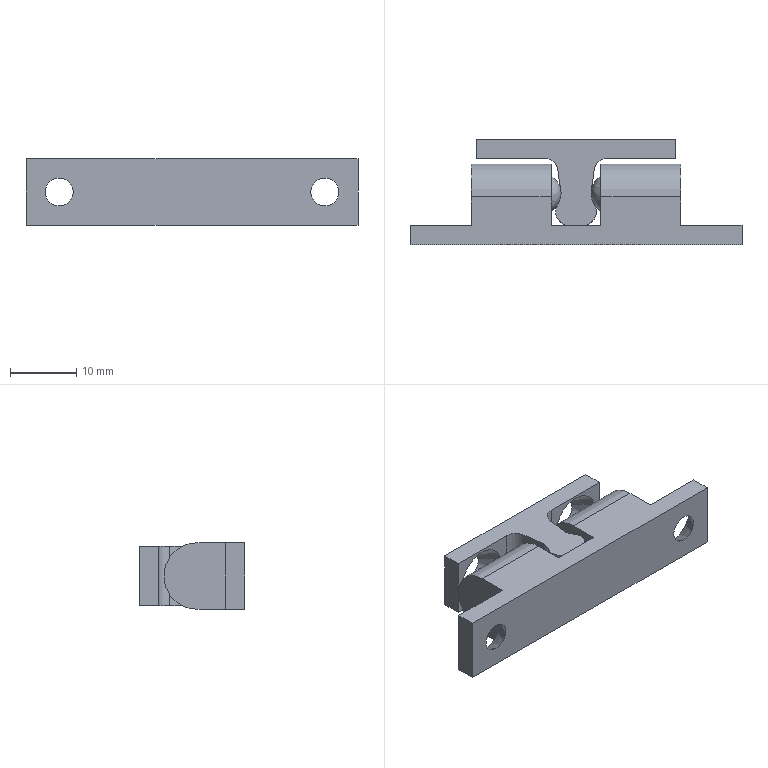Part | SolidWorks | features BaseBody 2 | 2 solids | 45 faces | box 50 x 15.9 x 10 mm | volume 4373 mm3 | plane 21 | cylinder 12 | cone 8 | spline 4 | commonest cylinder face diameters 6 x5 3.9 x3 4 x2 10 x2
STEP:
#1=CARTESIAN_POINT('',(-2.25,7.7,0.));
#2=VERTEX_POINT('',#1);
#3=CARTESIAN_POINT('',(-3.75,10.298,0.));
#4=VERTEX_POINT('',#3);
#5=CARTESIAN_POINT('',(-5.25,7.7,0.));
#6=DIRECTION('',(0.,0.,1.));
#7=DIRECTION('',(1.,0.,0.));
#8=AXIS2_PLACEMENT_3D('',#5,#6,#7);
#9=CIRCLE('',#8,3.);
#10=EDGE_CURVE('',#2,#4,#9,.T.);
#11=ORIENTED_EDGE('',*,*,#10,.F.);
#12=CARTESIAN_POINT('',(-3.75,5.102,0.));
#13=VERTEX_POINT('',#12);
#14=CARTESIAN_POINT('',(-5.25,7.7,0.));
#15=DIRECTION('',(0.,0.,-1.));
#16=DIRECTION('',(1.,0.,0.));
#17=AXIS2_PLACEMENT_3D('',#14,#15,#16);
#18=CIRCLE('',#17,3.);
#19=EDGE_CURVE('',#2,#13,#18,.T.);
#20=ORIENTED_EDGE('',*,*,#19,.T.);
#21=CARTESIAN_POINT('',(-3.75,7.7,0.));
#22=DIRECTION('',(-1.,0.,0.));
#23=DIRECTION('',(0.,0.,-1.));
#24=AXIS2_PLACEMENT_3D('',#21,#22,#23);
#25=CIRCLE('',#24,2.598);
#26=EDGE_CURVE('',#4,#13,#25,.T.);
#27=ORIENTED_EDGE('',*,*,#26,.F.);
#28=EDGE_LOOP('',(#11,#20,#27));
#29=FACE_OUTER_BOUND('',#28,.T.);
#30=CARTESIAN_POINT('',(-2.25,7.7,0.));
#31=CARTESIAN_POINT('',(-2.25,7.7,0.));
#32=CARTESIAN_POINT('',(-2.25,7.7,0.));
#33=CARTESIAN_POINT('',(-2.25,7.7,0.));
#34=CARTESIAN_POINT('',(-2.25,6.602,0.));
#35=CARTESIAN_POINT('',(-2.25,6.602,-2.196));
#36=CARTESIAN_POINT('',(-2.25,8.798,-2.196));
#37=CARTESIAN_POINT('',(-2.25,8.798,0.));
#38=CARTESIAN_POINT('',(-2.799,5.651,0.));
#39=CARTESIAN_POINT('',(-2.799,5.651,-4.098));
#40=CARTESIAN_POINT('',(-2.799,9.749,-4.098));
#41=CARTESIAN_POINT('',(-2.799,9.749,0.));
#42=CARTESIAN_POINT('',(-3.75,5.102,0.));
#43=CARTESIAN_POINT('',(-3.75,5.102,-5.196));
#44=CARTESIAN_POINT('',(-3.75,10.298,-5.196));
#45=CARTESIAN_POINT('',(-3.75,10.298,0.));
#46=(BOUNDED_SURFACE()B_SPLINE_SURFACE(3,3,((#30,#31,#32,#33),(#34,#35,#36,#37),(#38,#39,#40,#41),(#42,#43,#44,#45)),.UNSPECIFIED.,.F.,.F.,.F.)B_SPLINE_SURFACE_WITH_KNOTS((4,4),(4,4),(0.,1.),(0.,1.),.UNSPECIFIED.)GEOMETRIC_REPRESENTATION_ITEM()RATIONAL_B_SPLINE_SURFACE(((1.,0.3333,0.3333,1.),(0.9107,0.3036,0.3036,0.9107),(0.9107,0.3036,0.3036,0.9107),(1.,0.3333,0.3333,1.)))REPRESENTATION_ITEM('')SURFACE());
#47=ADVANCED_FACE('',(#29),#46,.T.);
#48=CARTESIAN_POINT('',(3.75,5.102,0.));
#49=VERTEX_POINT('',#48);
#50=CARTESIAN_POINT('',(3.75,10.298,0.));
#51=VERTEX_POINT('',#50);
#52=CARTESIAN_POINT('',(3.75,7.7,0.));
#53=DIRECTION('',(1.,0.,0.));
#54=DIRECTION('',(0.,0.,-1.));
#55=AXIS2_PLACEMENT_3D('',#52,#53,#54);
#56=CIRCLE('',#55,2.598);
#57=EDGE_CURVE('',#49,#51,#56,.T.);
#58=ORIENTED_EDGE('',*,*,#57,.F.);
#59=CARTESIAN_POINT('',(2.25,7.7,0.));
#60=VERTEX_POINT('',#59);
#61=CARTESIAN_POINT('',(5.25,7.7,0.));
#62=DIRECTION('',(0.,0.,-1.));
#63=DIRECTION('',(1.,0.,0.));
#64=AXIS2_PLACEMENT_3D('',#61,#62,#63);
#65=CIRCLE('',#64,3.);
#66=EDGE_CURVE('',#49,#60,#65,.T.);
#67=ORIENTED_EDGE('',*,*,#66,.T.);
#68=CARTESIAN_POINT('',(5.25,7.7,0.));
#69=DIRECTION('',(0.,0.,1.));
#70=DIRECTION('',(1.,0.,0.));
#71=AXIS2_PLACEMENT_3D('',#68,#69,#70);
#72=CIRCLE('',#71,3.);
#73=EDGE_CURVE('',#51,#60,#72,.T.);
#74=ORIENTED_EDGE('',*,*,#73,.F.);
#75=EDGE_LOOP('',(#58,#67,#74));
#76=FACE_OUTER_BOUND('',#75,.T.);
#77=CARTESIAN_POINT('',(3.75,5.102,0.));
#78=CARTESIAN_POINT('',(3.75,5.102,-5.196));
#79=CARTESIAN_POINT('',(3.75,10.298,-5.196));
#80=CARTESIAN_POINT('',(3.75,10.298,0.));
#81=CARTESIAN_POINT('',(2.799,5.651,0.));
#82=CARTESIAN_POINT('',(2.799,5.651,-4.098));
#83=CARTESIAN_POINT('',(2.799,9.749,-4.098));
#84=CARTESIAN_POINT('',(2.799,9.749,0.));
#85=CARTESIAN_POINT('',(2.25,6.602,0.));
#86=CARTESIAN_POINT('',(2.25,6.602,-2.196));
#87=CARTESIAN_POINT('',(2.25,8.798,-2.196));
#88=CARTESIAN_POINT('',(2.25,8.798,0.));
#89=CARTESIAN_POINT('',(2.25,7.7,0.));
#90=CARTESIAN_POINT('',(2.25,7.7,0.));
#91=CARTESIAN_POINT('',(2.25,7.7,0.));
#92=CARTESIAN_POINT('',(2.25,7.7,0.));
#93=(BOUNDED_SURFACE()B_SPLINE_SURFACE(3,3,((#77,#78,#79,#80),(#81,#82,#83,#84),(#85,#86,#87,#88),(#89,#90,#91,#92)),.UNSPECIFIED.,.F.,.F.,.T.)B_SPLINE_SURFACE_WITH_KNOTS((4,4),(4,4),(0.,1.),(0.,1.),.UNSPECIFIED.)GEOMETRIC_REPRESENTATION_ITEM()RATIONAL_B_SPLINE_SURFACE(((1.,0.3333,0.3333,1.),(0.9107,0.3036,0.3036,0.9107),(0.9107,0.3036,0.3036,0.9107),(1.,0.3333,0.3333,1.)))REPRESENTATION_ITEM('')SURFACE());
#94=ADVANCED_FACE('',(#76),#93,.T.);
#95=CARTESIAN_POINT('',(20.,0.,-2.1));
#96=VERTEX_POINT('',#95);
#97=CARTESIAN_POINT('',(20.,0.,2.1));
#98=VERTEX_POINT('',#97);
#99=CARTESIAN_POINT('',(20.,0.,0.));
#100=DIRECTION('',(0.,1.,0.));
#101=DIRECTION('',(0.,0.,1.));
#102=AXIS2_PLACEMENT_3D('',#99,#100,#101);
#103=CIRCLE('',#102,2.1);
#104=EDGE_CURVE('',#96,#98,#103,.T.);
#105=ORIENTED_EDGE('',*,*,#104,.F.);
#106=CARTESIAN_POINT('',(20.,2.9,-4.1));
#107=VERTEX_POINT('',#106);
#108=CARTESIAN_POINT('',(20.,2.9,-4.1));
#109=DIRECTION('',(0.,0.8232,-0.5677));
#110=VECTOR('',#109,1000.);
#111=LINE('',#108,#110);
#112=EDGE_CURVE('',#96,#107,#111,.T.);
#113=ORIENTED_EDGE('',*,*,#112,.T.);
#114=CARTESIAN_POINT('',(20.,2.9,4.1));
#115=VERTEX_POINT('',#114);
#116=CARTESIAN_POINT('',(20.,2.9,0.));
#117=DIRECTION('',(0.,-1.,0.));
#118=DIRECTION('',(0.,0.,1.));
#119=AXIS2_PLACEMENT_3D('',#116,#117,#118);
#120=CIRCLE('',#119,4.1);
#121=EDGE_CURVE('',#115,#107,#120,.T.);
#122=ORIENTED_EDGE('',*,*,#121,.F.);
#123=CARTESIAN_POINT('',(20.,2.9,4.1));
#124=DIRECTION('',(0.,0.8232,0.5677));
#125=VECTOR('',#124,1000.);
#126=LINE('',#123,#125);
#127=EDGE_CURVE('',#98,#115,#126,.T.);
#128=ORIENTED_EDGE('',*,*,#127,.F.);
#129=EDGE_LOOP('',(#105,#113,#122,#128));
#130=FACE_OUTER_BOUND('',#129,.T.);
#131=CARTESIAN_POINT('',(20.,2.9,0.));
#132=DIRECTION('',(0.,1.,0.));
#133=DIRECTION('',(0.,0.,1.));
#134=AXIS2_PLACEMENT_3D('',#131,#132,#133);
#135=CONICAL_SURFACE('',#134,4.1,0.6037);
#136=ADVANCED_FACE('',(#130),#135,.F.);
#137=CARTESIAN_POINT('',(-20.,0.,-2.1));
#138=VERTEX_POINT('',#137);
#139=CARTESIAN_POINT('',(-20.,0.,2.1));
#140=VERTEX_POINT('',#139);
#141=CARTESIAN_POINT('',(-20.,0.,0.));
#142=DIRECTION('',(0.,1.,0.));
#143=DIRECTION('',(0.,0.,1.));
#144=AXIS2_PLACEMENT_3D('',#141,#142,#143);
#145=CIRCLE('',#144,2.1);
#146=EDGE_CURVE('',#138,#140,#145,.T.);
#147=ORIENTED_EDGE('',*,*,#146,.F.);
#148=CARTESIAN_POINT('',(-20.,2.9,-4.1));
#149=VERTEX_POINT('',#148);
#150=CARTESIAN_POINT('',(-20.,2.9,-4.1));
#151=DIRECTION('',(0.,0.8232,-0.5677));
#152=VECTOR('',#151,1000.);
#153=LINE('',#150,#152);
#154=EDGE_CURVE('',#138,#149,#153,.T.);
#155=ORIENTED_EDGE('',*,*,#154,.T.);
#156=CARTESIAN_POINT('',(-20.,2.9,4.1));
#157=VERTEX_POINT('',#156);
#158=CARTESIAN_POINT('',(-20.,2.9,0.));
#159=DIRECTION('',(0.,-1.,0.));
#160=DIRECTION('',(0.,0.,1.));
#161=AXIS2_PLACEMENT_3D('',#158,#159,#160);
#162=CIRCLE('',#161,4.1);
#163=EDGE_CURVE('',#157,#149,#162,.T.);
#164=ORIENTED_EDGE('',*,*,#163,.F.);
#165=CARTESIAN_POINT('',(-20.,2.9,4.1));
#166=DIRECTION('',(0.,0.8232,0.5677));
#167=VECTOR('',#166,1000.);
#168=LINE('',#165,#167);
#169=EDGE_CURVE('',#140,#157,#168,.T.);
#170=ORIENTED_EDGE('',*,*,#169,.F.);
#171=EDGE_LOOP('',(#147,#155,#164,#170));
#172=FACE_OUTER_BOUND('',#171,.T.);
#173=CARTESIAN_POINT('',(-20.,2.9,0.));
#174=DIRECTION('',(0.,1.,0.));
#175=DIRECTION('',(0.,0.,1.));
#176=AXIS2_PLACEMENT_3D('',#173,#174,#175);
#177=CONICAL_SURFACE('',#176,4.1,0.6037);
#178=ADVANCED_FACE('',(#172),#177,.F.);
#179=CARTESIAN_POINT('',(25.,0.,5.));
#180=VERTEX_POINT('',#179);
#181=CARTESIAN_POINT('',(-25.,0.,5.));
#182=VERTEX_POINT('',#181);
#183=CARTESIAN_POINT('',(-25.,0.,5.));
#184=DIRECTION('',(-1.,0.,0.));
#185=VECTOR('',#184,1000.);
#186=LINE('',#183,#185);
#187=EDGE_CURVE('',#180,#182,#186,.T.);
#188=ORIENTED_EDGE('',*,*,#187,.T.);
#189=CARTESIAN_POINT('',(-25.,0.,-5.));
#190=VERTEX_POINT('',#189);
#191=CARTESIAN_POINT('',(-25.,0.,5.));
#192=DIRECTION('',(0.,0.,-1.));
#193=VECTOR('',#192,1000.);
#194=LINE('',#191,#193);
#195=EDGE_CURVE('',#182,#190,#194,.T.);
#196=ORIENTED_EDGE('',*,*,#195,.T.);
#197=CARTESIAN_POINT('',(25.,0.,-5.));
#198=VERTEX_POINT('',#197);
#199=CARTESIAN_POINT('',(-25.,0.,-5.));
#200=DIRECTION('',(1.,0.,0.));
#201=VECTOR('',#200,1000.);
#202=LINE('',#199,#201);
#203=EDGE_CURVE('',#190,#198,#202,.T.);
#204=ORIENTED_EDGE('',*,*,#203,.T.);
#205=CARTESIAN_POINT('',(25.,0.,5.));
#206=DIRECTION('',(0.,0.,1.));
#207=VECTOR('',#206,1000.);
#208=LINE('',#205,#207);
#209=EDGE_CURVE('',#198,#180,#208,.T.);
#210=ORIENTED_EDGE('',*,*,#209,.T.);
#211=EDGE_LOOP('',(#188,#196,#204,#210));
#212=FACE_OUTER_BOUND('',#211,.T.);
#213=CARTESIAN_POINT('',(20.,0.,0.));
#214=DIRECTION('',(0.,1.,0.));
#215=DIRECTION('',(0.,0.,1.));
#216=AXIS2_PLACEMENT_3D('',#213,#214,#215);
#217=CIRCLE('',#216,2.1);
#218=EDGE_CURVE('',#98,#96,#217,.T.);
#219=ORIENTED_EDGE('',*,*,#218,.T.);
#220=ORIENTED_EDGE('',*,*,#104,.T.);
#221=EDGE_LOOP('',(#219,#220));
#222=FACE_BOUND('',#221,.T.);
#223=CARTESIAN_POINT('',(-20.,0.,0.));
#224=DIRECTION('',(0.,1.,0.));
#225=DIRECTION('',(0.,0.,1.));
#226=AXIS2_PLACEMENT_3D('',#223,#224,#225);
#227=CIRCLE('',#226,2.1);
#228=EDGE_CURVE('',#140,#138,#227,.T.);
#229=ORIENTED_EDGE('',*,*,#228,.T.);
#230=ORIENTED_EDGE('',*,*,#146,.T.);
#231=EDGE_LOOP('',(#229,#230));
#232=FACE_BOUND('',#231,.T.);
#233=CARTESIAN_POINT('',(-25.,0.,5.));
#234=DIRECTION('',(0.,-1.,0.));
#235=DIRECTION('',(0.,0.,-1.));
#236=AXIS2_PLACEMENT_3D('',#233,#234,#235);
#237=PLANE('',#236);
#238=ADVANCED_FACE('',(#212,#222,#232),#237,.T.);
#239=CARTESIAN_POINT('',(-25.,2.9,5.));
#240=VERTEX_POINT('',#239);
#241=CARTESIAN_POINT('',(-25.,2.9,5.));
#242=DIRECTION('',(0.,1.,0.));
#243=VECTOR('',#242,1000.);
#244=LINE('',#241,#243);
#245=EDGE_CURVE('',#182,#240,#244,.T.);
#246=ORIENTED_EDGE('',*,*,#245,.T.);
#247=CARTESIAN_POINT('',(-25.,2.9,-5.));
#248=VERTEX_POINT('',#247);
#249=CARTESIAN_POINT('',(-25.,2.9,5.));
#250=DIRECTION('',(0.,0.,-1.));
#251=VECTOR('',#250,1000.);
#252=LINE('',#249,#251);
#253=EDGE_CURVE('',#240,#248,#252,.T.);
#254=ORIENTED_EDGE('',*,*,#253,.T.);
#255=CARTESIAN_POINT('',(-25.,2.9,-5.));
#256=DIRECTION('',(0.,-1.,0.));
#257=VECTOR('',#256,1000.);
#258=LINE('',#255,#257);
#259=EDGE_CURVE('',#248,#190,#258,.T.);
#260=ORIENTED_EDGE('',*,*,#259,.T.);
#261=ORIENTED_EDGE('',*,*,#195,.F.);
#262=EDGE_LOOP('',(#246,#254,#260,#261));
#263=FACE_OUTER_BOUND('',#262,.T.);
#264=CARTESIAN_POINT('',(-25.,2.9,5.));
#265=DIRECTION('',(-1.,0.,0.));
#266=DIRECTION('',(0.,0.,1.));
#267=AXIS2_PLACEMENT_3D('',#264,#265,#266);
#268=PLANE('',#267);
#269=ADVANCED_FACE('',(#263),#268,.T.);
#270=CARTESIAN_POINT('',(3.75,2.9,5.));
#271=VERTEX_POINT('',#270);
#272=CARTESIAN_POINT('',(-3.75,2.9,5.));
#273=VERTEX_POINT('',#272);
#274=CARTESIAN_POINT('',(0.,2.9,5.));
#275=DIRECTION('',(-1.,0.,0.));
#276=VECTOR('',#275,1000.);
#277=LINE('',#274,#276);
#278=EDGE_CURVE('',#271,#273,#277,.T.);
#279=ORIENTED_EDGE('',*,*,#278,.T.);
#280=CARTESIAN_POINT('',(-3.75,7.2,5.));
#281=VERTEX_POINT('',#280);
#282=CARTESIAN_POINT('',(-3.75,0.,5.));
#283=DIRECTION('',(0.,1.,0.));
#284=VECTOR('',#283,1000.);
#285=LINE('',#282,#284);
#286=EDGE_CURVE('',#273,#281,#285,.T.);
#287=ORIENTED_EDGE('',*,*,#286,.T.);
#288=CARTESIAN_POINT('',(-15.75,7.2,5.));
#289=VERTEX_POINT('',#288);
#290=CARTESIAN_POINT('',(0.,7.2,5.));
#291=DIRECTION('',(-1.,0.,0.));
#292=VECTOR('',#291,1000.);
#293=LINE('',#290,#292);
#294=EDGE_CURVE('',#281,#289,#293,.T.);
#295=ORIENTED_EDGE('',*,*,#294,.T.);
#296=CARTESIAN_POINT('',(-15.75,2.9,5.));
#297=VERTEX_POINT('',#296);
#298=CARTESIAN_POINT('',(-15.75,0.,5.));
#299=DIRECTION('',(0.,-1.,0.));
#300=VECTOR('',#299,1000.);
#301=LINE('',#298,#300);
#302=EDGE_CURVE('',#289,#297,#301,.T.);
#303=ORIENTED_EDGE('',*,*,#302,.T.);
#304=CARTESIAN_POINT('',(0.,2.9,5.));
#305=DIRECTION('',(-1.,0.,0.));
#306=VECTOR('',#305,1000.);
#307=LINE('',#304,#306);
#308=EDGE_CURVE('',#297,#240,#307,.T.);
#309=ORIENTED_EDGE('',*,*,#308,.T.);
#310=ORIENTED_EDGE('',*,*,#245,.F.);
#311=ORIENTED_EDGE('',*,*,#187,.F.);
#312=CARTESIAN_POINT('',(25.,2.9,5.));
#313=VERTEX_POINT('',#312);
#314=CARTESIAN_POINT('',(25.,0.,5.));
#315=DIRECTION('',(0.,1.,0.));
#316=VECTOR('',#315,1000.);
#317=LINE('',#314,#316);
#318=EDGE_CURVE('',#180,#313,#317,.T.);
#319=ORIENTED_EDGE('',*,*,#318,.T.);
#320=CARTESIAN_POINT('',(15.75,2.9,5.));
#321=VERTEX_POINT('',#320);
#322=CARTESIAN_POINT('',(0.,2.9,5.));
#323=DIRECTION('',(-1.,0.,0.));
#324=VECTOR('',#323,1000.);
#325=LINE('',#322,#324);
#326=EDGE_CURVE('',#313,#321,#325,.T.);
#327=ORIENTED_EDGE('',*,*,#326,.T.);
#328=CARTESIAN_POINT('',(15.75,7.2,5.));
#329=VERTEX_POINT('',#328);
#330=CARTESIAN_POINT('',(15.75,0.,5.));
#331=DIRECTION('',(0.,1.,0.));
#332=VECTOR('',#331,1000.);
#333=LINE('',#330,#332);
#334=EDGE_CURVE('',#321,#329,#333,.T.);
#335=ORIENTED_EDGE('',*,*,#334,.T.);
#336=CARTESIAN_POINT('',(3.75,7.2,5.));
#337=VERTEX_POINT('',#336);
#338=CARTESIAN_POINT('',(0.,7.2,5.));
#339=DIRECTION('',(-1.,0.,0.));
#340=VECTOR('',#339,1000.);
#341=LINE('',#338,#340);
#342=EDGE_CURVE('',#329,#337,#341,.T.);
#343=ORIENTED_EDGE('',*,*,#342,.T.);
#344=CARTESIAN_POINT('',(3.75,0.,5.));
#345=DIRECTION('',(0.,-1.,0.));
#346=VECTOR('',#345,1000.);
#347=LINE('',#344,#346);
#348=EDGE_CURVE('',#337,#271,#347,.T.);
#349=ORIENTED_EDGE('',*,*,#348,.T.);
#350=EDGE_LOOP('',(#279,#287,#295,#303,#309,#310,#311,#319,#327,#335,#343,#349));
#351=FACE_OUTER_BOUND('',#350,.T.);
#352=CARTESIAN_POINT('',(0.,0.,5.));
#353=DIRECTION('',(0.,0.,1.));
#354=DIRECTION('',(1.,0.,0.));
#355=AXIS2_PLACEMENT_3D('',#352,#353,#354);
#356=PLANE('',#355);
#357=ADVANCED_FACE('',(#351),#356,.T.);
#358=ORIENTED_EDGE('',*,*,#318,.F.);
#359=ORIENTED_EDGE('',*,*,#209,.F.);
#360=CARTESIAN_POINT('',(25.,2.9,-5.));
#361=VERTEX_POINT('',#360);
#362=CARTESIAN_POINT('',(25.,0.,-5.));
#363=DIRECTION('',(0.,1.,0.));
#364=VECTOR('',#363,1000.);
#365=LINE('',#362,#364);
#366=EDGE_CURVE('',#198,#361,#365,.T.);
#367=ORIENTED_EDGE('',*,*,#366,.T.);
#368=CARTESIAN_POINT('',(25.,2.9,5.));
#369=DIRECTION('',(0.,0.,1.));
#370=VECTOR('',#369,1000.);
#371=LINE('',#368,#370);
#372=EDGE_CURVE('',#361,#313,#371,.T.);
#373=ORIENTED_EDGE('',*,*,#372,.T.);
#374=EDGE_LOOP('',(#358,#359,#367,#373));
#375=FACE_OUTER_BOUND('',#374,.T.);
#376=CARTESIAN_POINT('',(25.,0.,5.));
#377=DIRECTION('',(1.,0.,0.));
#378=DIRECTION('',(0.,0.,-1.));
#379=AXIS2_PLACEMENT_3D('',#376,#377,#378);
#380=PLANE('',#379);
#381=ADVANCED_FACE('',(#375),#380,.T.);
#382=CARTESIAN_POINT('',(-3.75,2.9,-5.));
#383=VERTEX_POINT('',#382);
#384=CARTESIAN_POINT('',(-3.75,7.2,-5.));
#385=VERTEX_POINT('',#384);
#386=CARTESIAN_POINT('',(-3.75,0.,-5.));
#387=DIRECTION('',(0.,1.,0.));
#388=VECTOR('',#387,1000.);
#389=LINE('',#386,#388);
#390=EDGE_CURVE('',#383,#385,#389,.T.);
#391=ORIENTED_EDGE('',*,*,#390,.F.);
#392=CARTESIAN_POINT('',(3.75,2.9,-5.));
#393=VERTEX_POINT('',#392);
#394=CARTESIAN_POINT('',(0.,2.9,-5.));
#395=DIRECTION('',(-1.,0.,0.));
#396=VECTOR('',#395,1000.);
#397=LINE('',#394,#396);
#398=EDGE_CURVE('',#393,#383,#397,.T.);
#399=ORIENTED_EDGE('',*,*,#398,.F.);
#400=CARTESIAN_POINT('',(3.75,7.2,-5.));
#401=VERTEX_POINT('',#400);
#402=CARTESIAN_POINT('',(3.75,0.,-5.));
#403=DIRECTION('',(0.,-1.,0.));
#404=VECTOR('',#403,1000.);
#405=LINE('',#402,#404);
#406=EDGE_CURVE('',#401,#393,#405,.T.);
#407=ORIENTED_EDGE('',*,*,#406,.F.);
#408=CARTESIAN_POINT('',(15.75,7.2,-5.));
#409=VERTEX_POINT('',#408);
#410=CARTESIAN_POINT('',(0.,7.2,-5.));
#411=DIRECTION('',(-1.,0.,0.));
#412=VECTOR('',#411,1000.);
#413=LINE('',#410,#412);
#414=EDGE_CURVE('',#409,#401,#413,.T.);
#415=ORIENTED_EDGE('',*,*,#414,.F.);
#416=CARTESIAN_POINT('',(15.75,2.9,-5.));
#417=VERTEX_POINT('',#416);
#418=CARTESIAN_POINT('',(15.75,0.,-5.));
#419=DIRECTION('',(0.,1.,0.));
#420=VECTOR('',#419,1000.);
#421=LINE('',#418,#420);
#422=EDGE_CURVE('',#417,#409,#421,.T.);
#423=ORIENTED_EDGE('',*,*,#422,.F.);
#424=CARTESIAN_POINT('',(0.,2.9,-5.));
#425=DIRECTION('',(-1.,0.,0.));
#426=VECTOR('',#425,1000.);
#427=LINE('',#424,#426);
#428=EDGE_CURVE('',#361,#417,#427,.T.);
#429=ORIENTED_EDGE('',*,*,#428,.F.);
#430=ORIENTED_EDGE('',*,*,#366,.F.);
#431=ORIENTED_EDGE('',*,*,#203,.F.);
#432=ORIENTED_EDGE('',*,*,#259,.F.);
#433=CARTESIAN_POINT('',(-15.75,2.9,-5.));
#434=VERTEX_POINT('',#433);
#435=CARTESIAN_POINT('',(0.,2.9,-5.));
#436=DIRECTION('',(-1.,0.,0.));
#437=VECTOR('',#436,1000.);
#438=LINE('',#435,#437);
#439=EDGE_CURVE('',#434,#248,#438,.T.);
#440=ORIENTED_EDGE('',*,*,#439,.F.);
#441=CARTESIAN_POINT('',(-15.75,7.2,-5.));
#442=VERTEX_POINT('',#441);
#443=CARTESIAN_POINT('',(-15.75,0.,-5.));
#444=DIRECTION('',(0.,-1.,0.));
#445=VECTOR('',#444,1000.);
#446=LINE('',#443,#445);
#447=EDGE_CURVE('',#442,#434,#446,.T.);
#448=ORIENTED_EDGE('',*,*,#447,.F.);
#449=CARTESIAN_POINT('',(0.,7.2,-5.));
#450=DIRECTION('',(-1.,0.,0.));
#451=VECTOR('',#450,1000.);
#452=LINE('',#449,#451);
#453=EDGE_CURVE('',#385,#442,#452,.T.);
#454=ORIENTED_EDGE('',*,*,#453,.F.);
#455=EDGE_LOOP('',(#391,#399,#407,#415,#423,#429,#430,#431,#432,#440,#448,#454));
#456=FACE_OUTER_BOUND('',#455,.T.);
#457=CARTESIAN_POINT('',(0.,0.,-5.));
#458=DIRECTION('',(0.,0.,1.));
#459=DIRECTION('',(1.,0.,0.));
#460=AXIS2_PLACEMENT_3D('',#457,#458,#459);
#461=PLANE('',#460);
#462=ADVANCED_FACE('',(#456),#461,.F.);
#463=ORIENTED_EDGE('',*,*,#112,.F.);
#464=ORIENTED_EDGE('',*,*,#218,.F.);
#465=ORIENTED_EDGE('',*,*,#127,.T.);
#466=CARTESIAN_POINT('',(20.,2.9,0.));
#467=DIRECTION('',(0.,-1.,0.));
#468=DIRECTION('',(0.,0.,1.));
#469=AXIS2_PLACEMENT_3D('',#466,#467,#468);
#470=CIRCLE('',#469,4.1);
#471=EDGE_CURVE('',#107,#115,#470,.T.);
#472=ORIENTED_EDGE('',*,*,#471,.F.);
#473=EDGE_LOOP('',(#463,#464,#465,#472));
#474=FACE_OUTER_BOUND('',#473,.T.);
#475=CARTESIAN_POINT('',(20.,2.9,0.));
#476=DIRECTION('',(0.,1.,0.));
#477=DIRECTION('',(0.,0.,1.));
#478=AXIS2_PLACEMENT_3D('',#475,#476,#477);
#479=CONICAL_SURFACE('',#478,4.1,0.6037);
#480=ADVANCED_FACE('',(#474),#479,.F.);
#481=ORIENTED_EDGE('',*,*,#154,.F.);
#482=ORIENTED_EDGE('',*,*,#228,.F.);
#483=ORIENTED_EDGE('',*,*,#169,.T.);
#484=CARTESIAN_POINT('',(-20.,2.9,0.));
#485=DIRECTION('',(0.,-1.,0.));
#486=DIRECTION('',(0.,0.,1.));
#487=AXIS2_PLACEMENT_3D('',#484,#485,#486);
#488=CIRCLE('',#487,4.1);
#489=EDGE_CURVE('',#149,#157,#488,.T.);
#490=ORIENTED_EDGE('',*,*,#489,.F.);
#491=EDGE_LOOP('',(#481,#482,#483,#490));
#492=FACE_OUTER_BOUND('',#491,.T.);
#493=CARTESIAN_POINT('',(-20.,2.9,0.));
#494=DIRECTION('',(0.,1.,0.));
#495=DIRECTION('',(0.,0.,1.));
#496=AXIS2_PLACEMENT_3D('',#493,#494,#495);
#497=CONICAL_SURFACE('',#496,4.1,0.6037);
#498=ADVANCED_FACE('',(#492),#497,.F.);
#499=ORIENTED_EDGE('',*,*,#308,.F.);
#500=CARTESIAN_POINT('',(-15.75,2.9,5.));
#501=DIRECTION('',(0.,0.,-1.));
#502=VECTOR('',#501,1000.);
#503=LINE('',#500,#502);
#504=EDGE_CURVE('',#297,#434,#503,.T.);
#505=ORIENTED_EDGE('',*,*,#504,.T.);
#506=ORIENTED_EDGE('',*,*,#439,.T.);
#507=ORIENTED_EDGE('',*,*,#253,.F.);
#508=EDGE_LOOP('',(#499,#505,#506,#507));
#509=FACE_OUTER_BOUND('',#508,.T.);
#510=ORIENTED_EDGE('',*,*,#163,.T.);
#511=ORIENTED_EDGE('',*,*,#489,.T.);
#512=EDGE_LOOP('',(#510,#511));
#513=FACE_BOUND('',#512,.T.);
#514=CARTESIAN_POINT('',(-15.75,2.9,5.));
#515=DIRECTION('',(0.,1.,0.));
#516=DIRECTION('',(0.,0.,1.));
#517=AXIS2_PLACEMENT_3D('',#514,#515,#516);
#518=PLANE('',#517);
#519=ADVANCED_FACE('',(#509,#513),#518,.T.);
#520=CARTESIAN_POINT('',(-3.75,2.9,5.));
#521=DIRECTION('',(0.,0.,-1.));
#522=VECTOR('',#521,1000.);
#523=LINE('',#520,#522);
#524=EDGE_CURVE('',#273,#383,#523,.T.);
#525=ORIENTED_EDGE('',*,*,#524,.T.);
#526=ORIENTED_EDGE('',*,*,#390,.T.);
#527=CARTESIAN_POINT('',(-3.75,7.2,0.));
#528=DIRECTION('',(1.,0.,0.));
#529=DIRECTION('',(0.,0.,-1.));
#530=AXIS2_PLACEMENT_3D('',#527,#528,#529);
#531=CIRCLE('',#530,5.);
#532=EDGE_CURVE('',#385,#281,#531,.T.);
#533=ORIENTED_EDGE('',*,*,#532,.T.);
#534=ORIENTED_EDGE('',*,*,#286,.F.);
#535=EDGE_LOOP('',(#525,#526,#533,#534));
#536=FACE_OUTER_BOUND('',#535,.T.);
#537=ORIENTED_EDGE('',*,*,#26,.T.);
#538=CARTESIAN_POINT('',(-3.75,7.7,0.));
#539=DIRECTION('',(-1.,0.,0.));
#540=DIRECTION('',(0.,0.,-1.));
#541=AXIS2_PLACEMENT_3D('',#538,#539,#540);
#542=CIRCLE('',#541,2.598);
#543=EDGE_CURVE('',#13,#4,#542,.T.);
#544=ORIENTED_EDGE('',*,*,#543,.T.);
#545=EDGE_LOOP('',(#537,#544));
#546=FACE_BOUND('',#545,.T.);
#547=CARTESIAN_POINT('',(-3.75,2.9,5.));
#548=DIRECTION('',(1.,0.,0.));
#549=DIRECTION('',(0.,0.,-1.));
#550=AXIS2_PLACEMENT_3D('',#547,#548,#549);
#551=PLANE('',#550);
#552=ADVANCED_FACE('',(#536,#546),#551,.T.);
#553=ORIENTED_EDGE('',*,*,#278,.F.);
#554=CARTESIAN_POINT('',(3.75,2.9,5.));
#555=DIRECTION('',(0.,0.,-1.));
#556=VECTOR('',#555,1000.);
#557=LINE('',#554,#556);
#558=EDGE_CURVE('',#271,#393,#557,.T.);
#559=ORIENTED_EDGE('',*,*,#558,.T.);
#560=ORIENTED_EDGE('',*,*,#398,.T.);
#561=ORIENTED_EDGE('',*,*,#524,.F.);
#562=EDGE_LOOP('',(#553,#559,#560,#561));
#563=FACE_OUTER_BOUND('',#562,.T.);
#564=CARTESIAN_POINT('',(3.75,2.9,5.));
#565=DIRECTION('',(0.,1.,0.));
#566=DIRECTION('',(0.,0.,1.));
#567=AXIS2_PLACEMENT_3D('',#564,#565,#566);
#568=PLANE('',#567);
#569=ADVANCED_FACE('',(#563),#568,.T.);
#570=ORIENTED_EDGE('',*,*,#558,.F.);
#571=ORIENTED_EDGE('',*,*,#348,.F.);
#572=CARTESIAN_POINT('',(3.75,7.2,0.));
#573=DIRECTION('',(-1.,0.,0.));
#574=DIRECTION('',(0.,0.,-1.));
#575=AXIS2_PLACEMENT_3D('',#572,#573,#574);
#576=CIRCLE('',#575,5.);
#577=EDGE_CURVE('',#337,#401,#576,.T.);
#578=ORIENTED_EDGE('',*,*,#577,.T.);
#579=ORIENTED_EDGE('',*,*,#406,.T.);
#580=EDGE_LOOP('',(#570,#571,#578,#579));
#581=FACE_OUTER_BOUND('',#580,.T.);
#582=CARTESIAN_POINT('',(3.75,7.7,0.));
#583=DIRECTION('',(1.,0.,0.));
#584=DIRECTION('',(0.,0.,-1.));
#585=AXIS2_PLACEMENT_3D('',#582,#583,#584);
#586=CIRCLE('',#585,2.598);
#587=EDGE_CURVE('',#51,#49,#586,.T.);
#588=ORIENTED_EDGE('',*,*,#587,.T.);
#589=ORIENTED_EDGE('',*,*,#57,.T.);
#590=EDGE_LOOP('',(#588,#589));
#591=FACE_BOUND('',#590,.T.);
#592=CARTESIAN_POINT('',(3.75,12.2,5.));
#593=DIRECTION('',(-1.,0.,0.));
#594=DIRECTION('',(0.,-1.,0.));
#595=AXIS2_PLACEMENT_3D('',#592,#593,#594);
#596=PLANE('',#595);
#597=ADVANCED_FACE('',(#581,#591),#596,.T.);
#598=CARTESIAN_POINT('',(15.75,7.2,0.));
#599=DIRECTION('',(-1.,0.,0.));
#600=DIRECTION('',(0.,0.,-1.));
#601=AXIS2_PLACEMENT_3D('',#598,#599,#600);
#602=CIRCLE('',#601,5.);
#603=EDGE_CURVE('',#329,#409,#602,.T.);
#604=ORIENTED_EDGE('',*,*,#603,.T.);
#605=ORIENTED_EDGE('',*,*,#414,.T.);
#606=ORIENTED_EDGE('',*,*,#577,.F.);
#607=ORIENTED_EDGE('',*,*,#342,.F.);
#608=EDGE_LOOP('',(#604,#605,#606,#607));
#609=FACE_OUTER_BOUND('',#608,.T.);
#610=CARTESIAN_POINT('',(50.,7.2,0.));
#611=DIRECTION('',(1.,0.,0.));
#612=DIRECTION('',(0.,0.,-1.));
#613=AXIS2_PLACEMENT_3D('',#610,#611,#612);
#614=CYLINDRICAL_SURFACE('',#613,5.);
#615=ADVANCED_FACE('',(#609),#614,.T.);
#616=CARTESIAN_POINT('',(15.75,2.9,5.));
#617=DIRECTION('',(0.,0.,-1.));
#618=VECTOR('',#617,1000.);
#619=LINE('',#616,#618);
#620=EDGE_CURVE('',#321,#417,#619,.T.);
#621=ORIENTED_EDGE('',*,*,#620,.T.);
#622=ORIENTED_EDGE('',*,*,#422,.T.);
#623=ORIENTED_EDGE('',*,*,#603,.F.);
#624=ORIENTED_EDGE('',*,*,#334,.F.);
#625=EDGE_LOOP('',(#621,#622,#623,#624));
#626=FACE_OUTER_BOUND('',#625,.T.);
#627=CARTESIAN_POINT('',(15.75,2.9,5.));
#628=DIRECTION('',(1.,0.,0.));
#629=DIRECTION('',(0.,0.,-1.));
#630=AXIS2_PLACEMENT_3D('',#627,#628,#629);
#631=PLANE('',#630);
#632=ADVANCED_FACE('',(#626),#631,.T.);
#633=ORIENTED_EDGE('',*,*,#326,.F.);
#634=ORIENTED_EDGE('',*,*,#372,.F.);
#635=ORIENTED_EDGE('',*,*,#428,.T.);
#636=ORIENTED_EDGE('',*,*,#620,.F.);
#637=EDGE_LOOP('',(#633,#634,#635,#636));
#638=FACE_OUTER_BOUND('',#637,.T.);
#639=ORIENTED_EDGE('',*,*,#121,.T.);
#640=ORIENTED_EDGE('',*,*,#471,.T.);
#641=EDGE_LOOP('',(#639,#640));
#642=FACE_BOUND('',#641,.T.);
#643=CARTESIAN_POINT('',(25.,2.9,5.));
#644=DIRECTION('',(0.,1.,0.));
#645=DIRECTION('',(-1.,0.,0.));
#646=AXIS2_PLACEMENT_3D('',#643,#644,#645);
#647=PLANE('',#646);
#648=ADVANCED_FACE('',(#638,#642),#647,.T.);
#649=ORIENTED_EDGE('',*,*,#504,.F.);
#650=ORIENTED_EDGE('',*,*,#302,.F.);
#651=CARTESIAN_POINT('',(-15.75,7.2,0.));
#652=DIRECTION('',(-1.,0.,0.));
#653=DIRECTION('',(0.,0.,-1.));
#654=AXIS2_PLACEMENT_3D('',#651,#652,#653);
#655=CIRCLE('',#654,5.);
#656=EDGE_CURVE('',#289,#442,#655,.T.);
#657=ORIENTED_EDGE('',*,*,#656,.T.);
#658=ORIENTED_EDGE('',*,*,#447,.T.);
#659=EDGE_LOOP('',(#649,#650,#657,#658));
#660=FACE_OUTER_BOUND('',#659,.T.);
#661=CARTESIAN_POINT('',(-15.75,12.2,5.));
#662=DIRECTION('',(-1.,0.,0.));
#663=DIRECTION('',(0.,0.,1.));
#664=AXIS2_PLACEMENT_3D('',#661,#662,#663);
#665=PLANE('',#664);
#666=ADVANCED_FACE('',(#660),#665,.T.);
#667=ORIENTED_EDGE('',*,*,#656,.F.);
#668=ORIENTED_EDGE('',*,*,#294,.F.);
#669=ORIENTED_EDGE('',*,*,#532,.F.);
#670=ORIENTED_EDGE('',*,*,#453,.T.);
#671=EDGE_LOOP('',(#667,#668,#669,#670));
#672=FACE_OUTER_BOUND('',#671,.T.);
#673=CARTESIAN_POINT('',(50.,7.2,0.));
#674=DIRECTION('',(1.,0.,0.));
#675=DIRECTION('',(0.,0.,-1.));
#676=AXIS2_PLACEMENT_3D('',#673,#674,#675);
#677=CYLINDRICAL_SURFACE('',#676,5.);
#678=ADVANCED_FACE('',(#672),#677,.T.);
#679=ORIENTED_EDGE('',*,*,#19,.F.);
#680=ORIENTED_EDGE('',*,*,#10,.T.);
#681=ORIENTED_EDGE('',*,*,#543,.F.);
#682=EDGE_LOOP('',(#679,#680,#681));
#683=FACE_OUTER_BOUND('',#682,.T.);
#684=CARTESIAN_POINT('',(-2.25,7.7,0.));
#685=CARTESIAN_POINT('',(-2.25,7.7,0.));
#686=CARTESIAN_POINT('',(-2.25,7.7,0.));
#687=CARTESIAN_POINT('',(-2.25,7.7,0.));
#688=CARTESIAN_POINT('',(-2.25,8.798,0.));
#689=CARTESIAN_POINT('',(-2.25,8.798,2.196));
#690=CARTESIAN_POINT('',(-2.25,6.602,2.196));
#691=CARTESIAN_POINT('',(-2.25,6.602,0.));
#692=CARTESIAN_POINT('',(-2.799,9.749,0.));
#693=CARTESIAN_POINT('',(-2.799,9.749,4.098));
#694=CARTESIAN_POINT('',(-2.799,5.651,4.098));
#695=CARTESIAN_POINT('',(-2.799,5.651,0.));
#696=CARTESIAN_POINT('',(-3.75,10.298,0.));
#697=CARTESIAN_POINT('',(-3.75,10.298,5.196));
#698=CARTESIAN_POINT('',(-3.75,5.102,5.196));
#699=CARTESIAN_POINT('',(-3.75,5.102,0.));
#700=(BOUNDED_SURFACE()B_SPLINE_SURFACE(3,3,((#684,#685,#686,#687),(#688,#689,#690,#691),(#692,#693,#694,#695),(#696,#697,#698,#699)),.UNSPECIFIED.,.F.,.F.,.F.)B_SPLINE_SURFACE_WITH_KNOTS((4,4),(4,4),(0.,1.),(0.,1.),.UNSPECIFIED.)GEOMETRIC_REPRESENTATION_ITEM()RATIONAL_B_SPLINE_SURFACE(((1.,0.3333,0.3333,1.),(0.9107,0.3036,0.3036,0.9107),(0.9107,0.3036,0.3036,0.9107),(1.,0.3333,0.3333,1.)))REPRESENTATION_ITEM('')SURFACE());
#701=ADVANCED_FACE('',(#683),#700,.T.);
#702=ORIENTED_EDGE('',*,*,#66,.F.);
#703=ORIENTED_EDGE('',*,*,#587,.F.);
#704=ORIENTED_EDGE('',*,*,#73,.T.);
#705=EDGE_LOOP('',(#702,#703,#704));
#706=FACE_OUTER_BOUND('',#705,.T.);
#707=CARTESIAN_POINT('',(3.75,10.298,0.));
#708=CARTESIAN_POINT('',(3.75,10.298,5.196));
#709=CARTESIAN_POINT('',(3.75,5.102,5.196));
#710=CARTESIAN_POINT('',(3.75,5.102,0.));
#711=CARTESIAN_POINT('',(2.799,9.749,0.));
#712=CARTESIAN_POINT('',(2.799,9.749,4.098));
#713=CARTESIAN_POINT('',(2.799,5.651,4.098));
#714=CARTESIAN_POINT('',(2.799,5.651,0.));
#715=CARTESIAN_POINT('',(2.25,8.798,0.));
#716=CARTESIAN_POINT('',(2.25,8.798,2.196));
#717=CARTESIAN_POINT('',(2.25,6.602,2.196));
#718=CARTESIAN_POINT('',(2.25,6.602,0.));
#719=CARTESIAN_POINT('',(2.25,7.7,0.));
#720=CARTESIAN_POINT('',(2.25,7.7,0.));
#721=CARTESIAN_POINT('',(2.25,7.7,0.));
#722=CARTESIAN_POINT('',(2.25,7.7,0.));
#723=(BOUNDED_SURFACE()B_SPLINE_SURFACE(3,3,((#707,#708,#709,#710),(#711,#712,#713,#714),(#715,#716,#717,#718),(#719,#720,#721,#722)),.UNSPECIFIED.,.F.,.F.,.F.)B_SPLINE_SURFACE_WITH_KNOTS((4,4),(4,4),(0.,1.),(0.,1.),.UNSPECIFIED.)GEOMETRIC_REPRESENTATION_ITEM()RATIONAL_B_SPLINE_SURFACE(((1.,0.3333,0.3333,1.),(0.9107,0.3036,0.3036,0.9107),(0.9107,0.3036,0.3036,0.9107),(1.,0.3333,0.3333,1.)))REPRESENTATION_ITEM('')SURFACE());
#724=ADVANCED_FACE('',(#706),#723,.T.);
#725=CLOSED_SHELL('',(#47,#94,#136,#178,#238,#269,#357,#381,#462,#480,#498,#519,#552,#569,#597,#615,#632,#648,#666,#678,#701,#724));
#726=MANIFOLD_SOLID_BREP('',#725);
#727=CARTESIAN_POINT('',(10.,15.9,2.1));
#728=VERTEX_POINT('',#727);
#729=CARTESIAN_POINT('',(10.,15.9,-2.1));
#730=VERTEX_POINT('',#729);
#731=CARTESIAN_POINT('',(10.,15.9,0.));
#732=DIRECTION('',(0.,-1.,0.));
#733=DIRECTION('',(0.,0.,-1.));
#734=AXIS2_PLACEMENT_3D('',#731,#732,#733);
#735=CIRCLE('',#734,2.1);
#736=EDGE_CURVE('',#728,#730,#735,.T.);
#737=ORIENTED_EDGE('',*,*,#736,.F.);
#738=CARTESIAN_POINT('',(10.,13.,4.1));
#739=VERTEX_POINT('',#738);
#740=CARTESIAN_POINT('',(10.,13.,4.1));
#741=DIRECTION('',(0.,-0.8232,0.5677));
#742=VECTOR('',#741,1000.);
#743=LINE('',#740,#742);
#744=EDGE_CURVE('',#728,#739,#743,.T.);
#745=ORIENTED_EDGE('',*,*,#744,.T.);
#746=CARTESIAN_POINT('',(10.,13.,-4.1));
#747=VERTEX_POINT('',#746);
#748=CARTESIAN_POINT('',(10.,13.,0.));
#749=DIRECTION('',(0.,1.,0.));
#750=DIRECTION('',(0.,0.,-1.));
#751=AXIS2_PLACEMENT_3D('',#748,#749,#750);
#752=CIRCLE('',#751,4.1);
#753=EDGE_CURVE('',#747,#739,#752,.T.);
#754=ORIENTED_EDGE('',*,*,#753,.F.);
#755=CARTESIAN_POINT('',(10.,13.,-4.1));
#756=DIRECTION('',(0.,-0.8232,-0.5677));
#757=VECTOR('',#756,1000.);
#758=LINE('',#755,#757);
#759=EDGE_CURVE('',#730,#747,#758,.T.);
#760=ORIENTED_EDGE('',*,*,#759,.F.);
#761=EDGE_LOOP('',(#737,#745,#754,#760));
#762=FACE_OUTER_BOUND('',#761,.T.);
#763=CARTESIAN_POINT('',(10.,13.,0.));
#764=DIRECTION('',(0.,-1.,0.));
#765=DIRECTION('',(0.,0.,-1.));
#766=AXIS2_PLACEMENT_3D('',#763,#764,#765);
#767=CONICAL_SURFACE('',#766,4.1,0.6037);
#768=ADVANCED_FACE('',(#762),#767,.F.);
#769=CARTESIAN_POINT('',(-10.,15.9,2.1));
#770=VERTEX_POINT('',#769);
#771=CARTESIAN_POINT('',(-10.,15.9,-2.1));
#772=VERTEX_POINT('',#771);
#773=CARTESIAN_POINT('',(-10.,15.9,0.));
#774=DIRECTION('',(0.,-1.,0.));
#775=DIRECTION('',(0.,0.,-1.));
#776=AXIS2_PLACEMENT_3D('',#773,#774,#775);
#777=CIRCLE('',#776,2.1);
#778=EDGE_CURVE('',#770,#772,#777,.T.);
#779=ORIENTED_EDGE('',*,*,#778,.F.);
#780=CARTESIAN_POINT('',(-10.,13.,4.1));
#781=VERTEX_POINT('',#780);
#782=CARTESIAN_POINT('',(-10.,13.,4.1));
#783=DIRECTION('',(0.,-0.8232,0.5677));
#784=VECTOR('',#783,1000.);
#785=LINE('',#782,#784);
#786=EDGE_CURVE('',#770,#781,#785,.T.);
#787=ORIENTED_EDGE('',*,*,#786,.T.);
#788=CARTESIAN_POINT('',(-10.,13.,-4.1));
#789=VERTEX_POINT('',#788);
#790=CARTESIAN_POINT('',(-10.,13.,0.));
#791=DIRECTION('',(0.,1.,0.));
#792=DIRECTION('',(0.,0.,-1.));
#793=AXIS2_PLACEMENT_3D('',#790,#791,#792);
#794=CIRCLE('',#793,4.1);
#795=EDGE_CURVE('',#789,#781,#794,.T.);
#796=ORIENTED_EDGE('',*,*,#795,.F.);
#797=CARTESIAN_POINT('',(-10.,13.,-4.1));
#798=DIRECTION('',(0.,-0.8232,-0.5677));
#799=VECTOR('',#798,1000.);
#800=LINE('',#797,#799);
#801=EDGE_CURVE('',#772,#789,#800,.T.);
#802=ORIENTED_EDGE('',*,*,#801,.F.);
#803=EDGE_LOOP('',(#779,#787,#796,#802));
#804=FACE_OUTER_BOUND('',#803,.T.);
#805=CARTESIAN_POINT('',(-10.,13.,0.));
#806=DIRECTION('',(0.,-1.,0.));
#807=DIRECTION('',(0.,0.,-1.));
#808=AXIS2_PLACEMENT_3D('',#805,#806,#807);
#809=CONICAL_SURFACE('',#808,4.1,0.6037);
#810=ADVANCED_FACE('',(#804),#809,.F.);
#811=CARTESIAN_POINT('',(2.536,3.581,-4.5));
#812=VERTEX_POINT('',#811);
#813=CARTESIAN_POINT('',(3.09,4.942,-4.5));
#814=VERTEX_POINT('',#813);
#815=CARTESIAN_POINT('',(1.14,4.942,-4.5));
#816=DIRECTION('',(0.,0.,1.));
#817=DIRECTION('',(1.,0.,0.));
#818=AXIS2_PLACEMENT_3D('',#815,#816,#817);
#819=CIRCLE('',#818,1.95);
#820=EDGE_CURVE('',#812,#814,#819,.T.);
#821=ORIENTED_EDGE('',*,*,#820,.T.);
#822=CARTESIAN_POINT('',(3.09,4.942,4.5));
#823=VERTEX_POINT('',#822);
#824=CARTESIAN_POINT('',(3.09,4.942,4.5));
#825=DIRECTION('',(0.,0.,1.));
#826=VECTOR('',#825,1000.);
#827=LINE('',#824,#826);
#828=EDGE_CURVE('',#814,#823,#827,.T.);
#829=ORIENTED_EDGE('',*,*,#828,.T.);
#830=CARTESIAN_POINT('',(2.536,3.581,4.5));
#831=VERTEX_POINT('',#830);
#832=CARTESIAN_POINT('',(1.14,4.942,4.5));
#833=DIRECTION('',(0.,0.,1.));
#834=DIRECTION('',(1.,0.,0.));
#835=AXIS2_PLACEMENT_3D('',#832,#833,#834);
#836=CIRCLE('',#835,1.95);
#837=EDGE_CURVE('',#831,#823,#836,.T.);
#838=ORIENTED_EDGE('',*,*,#837,.F.);
#839=CARTESIAN_POINT('',(2.536,3.581,4.5));
#840=DIRECTION('',(0.,0.,-1.));
#841=VECTOR('',#840,1000.);
#842=LINE('',#839,#841);
#843=EDGE_CURVE('',#831,#812,#842,.T.);
#844=ORIENTED_EDGE('',*,*,#843,.T.);
#845=EDGE_LOOP('',(#821,#829,#838,#844));
#846=FACE_OUTER_BOUND('',#845,.T.);
#847=CARTESIAN_POINT('',(1.14,4.942,4.5));
#848=DIRECTION('',(0.,0.,1.));
#849=DIRECTION('',(1.,0.,0.));
#850=AXIS2_PLACEMENT_3D('',#847,#848,#849);
#851=CYLINDRICAL_SURFACE('',#850,1.95);
#852=ADVANCED_FACE('',(#846),#851,.T.);
#853=CARTESIAN_POINT('',(-2.282,8.138,-4.5));
#854=VERTEX_POINT('',#853);
#855=CARTESIAN_POINT('',(-2.25,7.7,-4.5));
#856=VERTEX_POINT('',#855);
#857=CARTESIAN_POINT('',(-5.25,7.7,-4.5));
#858=DIRECTION('',(0.,0.,-1.));
#859=DIRECTION('',(1.,0.,0.));
#860=AXIS2_PLACEMENT_3D('',#857,#858,#859);
#861=CIRCLE('',#860,3.);
#862=EDGE_CURVE('',#854,#856,#861,.T.);
#863=ORIENTED_EDGE('',*,*,#862,.T.);
#864=CARTESIAN_POINT('',(-2.25,7.7,4.5));
#865=VERTEX_POINT('',#864);
#866=CARTESIAN_POINT('',(-2.25,7.7,4.5));
#867=DIRECTION('',(0.,0.,1.));
#868=VECTOR('',#867,1000.);
#869=LINE('',#866,#868);
#870=EDGE_CURVE('',#856,#865,#869,.T.);
#871=ORIENTED_EDGE('',*,*,#870,.T.);
#872=CARTESIAN_POINT('',(-2.282,8.138,4.5));
#873=VERTEX_POINT('',#872);
#874=CARTESIAN_POINT('',(-5.25,7.7,4.5));
#875=DIRECTION('',(0.,0.,-1.));
#876=DIRECTION('',(1.,0.,0.));
#877=AXIS2_PLACEMENT_3D('',#874,#875,#876);
#878=CIRCLE('',#877,3.);
#879=EDGE_CURVE('',#873,#865,#878,.T.);
#880=ORIENTED_EDGE('',*,*,#879,.F.);
#881=CARTESIAN_POINT('',(-2.282,8.138,4.5));
#882=DIRECTION('',(0.,0.,1.));
#883=VECTOR('',#882,1000.);
#884=LINE('',#881,#883);
#885=EDGE_CURVE('',#854,#873,#884,.T.);
#886=ORIENTED_EDGE('',*,*,#885,.F.);
#887=EDGE_LOOP('',(#863,#871,#880,#886));
#888=FACE_OUTER_BOUND('',#887,.T.);
#889=CARTESIAN_POINT('',(-5.25,7.7,4.5));
#890=DIRECTION('',(0.,0.,1.));
#891=DIRECTION('',(1.,0.,0.));
#892=AXIS2_PLACEMENT_3D('',#889,#890,#891);
#893=CYLINDRICAL_SURFACE('',#892,3.);
#894=ADVANCED_FACE('',(#888),#893,.F.);
#895=CARTESIAN_POINT('',(-15.,15.9,4.5));
#896=VERTEX_POINT('',#895);
#897=CARTESIAN_POINT('',(15.,15.9,4.5));
#898=VERTEX_POINT('',#897);
#899=CARTESIAN_POINT('',(15.,15.9,4.5));
#900=DIRECTION('',(1.,0.,0.));
#901=VECTOR('',#900,1000.);
#902=LINE('',#899,#901);
#903=EDGE_CURVE('',#896,#898,#902,.T.);
#904=ORIENTED_EDGE('',*,*,#903,.T.);
#905=CARTESIAN_POINT('',(15.,15.9,-4.5));
#906=VERTEX_POINT('',#905);
#907=CARTESIAN_POINT('',(15.,15.9,4.5));
#908=DIRECTION('',(0.,0.,-1.));
#909=VECTOR('',#908,1000.);
#910=LINE('',#907,#909);
#911=EDGE_CURVE('',#898,#906,#910,.T.);
#912=ORIENTED_EDGE('',*,*,#911,.T.);
#913=CARTESIAN_POINT('',(-15.,15.9,-4.5));
#914=VERTEX_POINT('',#913);
#915=CARTESIAN_POINT('',(15.,15.9,-4.5));
#916=DIRECTION('',(-1.,0.,0.));
#917=VECTOR('',#916,1000.);
#918=LINE('',#915,#917);
#919=EDGE_CURVE('',#906,#914,#918,.T.);
#920=ORIENTED_EDGE('',*,*,#919,.T.);
#921=CARTESIAN_POINT('',(-15.,15.9,4.5));
#922=DIRECTION('',(0.,0.,1.));
#923=VECTOR('',#922,1000.);
#924=LINE('',#921,#923);
#925=EDGE_CURVE('',#914,#896,#924,.T.);
#926=ORIENTED_EDGE('',*,*,#925,.T.);
#927=EDGE_LOOP('',(#904,#912,#920,#926));
#928=FACE_OUTER_BOUND('',#927,.T.);
#929=CARTESIAN_POINT('',(10.,15.9,0.));
#930=DIRECTION('',(0.,-1.,0.));
#931=DIRECTION('',(0.,0.,-1.));
#932=AXIS2_PLACEMENT_3D('',#929,#930,#931);
#933=CIRCLE('',#932,2.1);
#934=EDGE_CURVE('',#730,#728,#933,.T.);
#935=ORIENTED_EDGE('',*,*,#934,.T.);
#936=ORIENTED_EDGE('',*,*,#736,.T.);
#937=EDGE_LOOP('',(#935,#936));
#938=FACE_BOUND('',#937,.T.);
#939=CARTESIAN_POINT('',(-10.,15.9,0.));
#940=DIRECTION('',(0.,-1.,0.));
#941=DIRECTION('',(0.,0.,-1.));
#942=AXIS2_PLACEMENT_3D('',#939,#940,#941);
#943=CIRCLE('',#942,2.1);
#944=EDGE_CURVE('',#772,#770,#943,.T.);
#945=ORIENTED_EDGE('',*,*,#944,.T.);
#946=ORIENTED_EDGE('',*,*,#778,.T.);
#947=EDGE_LOOP('',(#945,#946));
#948=FACE_BOUND('',#947,.T.);
#949=CARTESIAN_POINT('',(15.,15.9,4.5));
#950=DIRECTION('',(0.,1.,0.));
#951=DIRECTION('',(0.,0.,1.));
#952=AXIS2_PLACEMENT_3D('',#949,#950,#951);
#953=PLANE('',#952);
#954=ADVANCED_FACE('',(#928,#938,#948),#953,.T.);
#955=CARTESIAN_POINT('',(15.,13.,4.5));
#956=VERTEX_POINT('',#955);
#957=CARTESIAN_POINT('',(15.,13.,4.5));
#958=DIRECTION('',(0.,-1.,0.));
#959=VECTOR('',#958,1000.);
#960=LINE('',#957,#959);
#961=EDGE_CURVE('',#898,#956,#960,.T.);
#962=ORIENTED_EDGE('',*,*,#961,.T.);
#963=CARTESIAN_POINT('',(15.,13.,-4.5));
#964=VERTEX_POINT('',#963);
#965=CARTESIAN_POINT('',(15.,13.,4.5));
#966=DIRECTION('',(0.,0.,-1.));
#967=VECTOR('',#966,1000.);
#968=LINE('',#965,#967);
#969=EDGE_CURVE('',#956,#964,#968,.T.);
#970=ORIENTED_EDGE('',*,*,#969,.T.);
#971=CARTESIAN_POINT('',(15.,13.,-4.5));
#972=DIRECTION('',(0.,1.,0.));
#973=VECTOR('',#972,1000.);
#974=LINE('',#971,#973);
#975=EDGE_CURVE('',#964,#906,#974,.T.);
#976=ORIENTED_EDGE('',*,*,#975,.T.);
#977=ORIENTED_EDGE('',*,*,#911,.F.);
#978=EDGE_LOOP('',(#962,#970,#976,#977));
#979=FACE_OUTER_BOUND('',#978,.T.);
#980=CARTESIAN_POINT('',(15.,13.,4.5));
#981=DIRECTION('',(1.,0.,0.));
#982=DIRECTION('',(0.,0.,-1.));
#983=AXIS2_PLACEMENT_3D('',#980,#981,#982);
#984=PLANE('',#983);
#985=ADVANCED_FACE('',(#979),#984,.T.);
#986=ORIENTED_EDGE('',*,*,#961,.F.);
#987=ORIENTED_EDGE('',*,*,#903,.F.);
#988=CARTESIAN_POINT('',(-15.,13.,4.5));
#989=VERTEX_POINT('',#988);
#990=CARTESIAN_POINT('',(-15.,0.,4.5));
#991=DIRECTION('',(0.,-1.,0.));
#992=VECTOR('',#991,1000.);
#993=LINE('',#990,#992);
#994=EDGE_CURVE('',#896,#989,#993,.T.);
#995=ORIENTED_EDGE('',*,*,#994,.T.);
#996=CARTESIAN_POINT('',(-4.726,13.,4.5));
#997=VERTEX_POINT('',#996);
#998=CARTESIAN_POINT('',(0.,13.,4.5));
#999=DIRECTION('',(1.,0.,0.));
#1000=VECTOR('',#999,1000.);
#1001=LINE('',#998,#1000);
#1002=EDGE_CURVE('',#989,#997,#1001,.T.);
#1003=ORIENTED_EDGE('',*,*,#1002,.T.);
#1004=CARTESIAN_POINT('',(-2.748,11.292,4.5));
#1005=VERTEX_POINT('',#1004);
#1006=CARTESIAN_POINT('',(-4.726,11.,4.5));
#1007=DIRECTION('',(0.,0.,-1.));
#1008=DIRECTION('',(1.,0.,0.));
#1009=AXIS2_PLACEMENT_3D('',#1006,#1007,#1008);
#1010=CIRCLE('',#1009,2.);
#1011=EDGE_CURVE('',#997,#1005,#1010,.T.);
#1012=ORIENTED_EDGE('',*,*,#1011,.T.);
#1013=CARTESIAN_POINT('',(-2.748,11.292,4.5));
#1014=DIRECTION('',(0.1461,-0.9893,0.));
#1015=VECTOR('',#1014,1000.);
#1016=LINE('',#1013,#1015);
#1017=EDGE_CURVE('',#1005,#873,#1016,.T.);
#1018=ORIENTED_EDGE('',*,*,#1017,.T.);
#1019=ORIENTED_EDGE('',*,*,#879,.T.);
#1020=CARTESIAN_POINT('',(-2.759,6.028,4.5));
#1021=VERTEX_POINT('',#1020);
#1022=CARTESIAN_POINT('',(-5.25,7.7,4.5));
#1023=DIRECTION('',(0.,0.,-1.));
#1024=DIRECTION('',(1.,0.,0.));
#1025=AXIS2_PLACEMENT_3D('',#1022,#1023,#1024);
#1026=CIRCLE('',#1025,3.);
#1027=EDGE_CURVE('',#865,#1021,#1026,.T.);
#1028=ORIENTED_EDGE('',*,*,#1027,.T.);
#1029=CARTESIAN_POINT('',(-2.536,3.581,4.5));
#1030=VERTEX_POINT('',#1029);
#1031=CARTESIAN_POINT('',(-1.14,4.942,4.5));
#1032=DIRECTION('',(0.,0.,1.));
#1033=DIRECTION('',(1.,0.,0.));
#1034=AXIS2_PLACEMENT_3D('',#1031,#1032,#1033);
#1035=CIRCLE('',#1034,1.95);
#1036=EDGE_CURVE('',#1021,#1030,#1035,.T.);
#1037=ORIENTED_EDGE('',*,*,#1036,.T.);
#1038=CARTESIAN_POINT('',(0.,2.7,4.5));
#1039=VERTEX_POINT('',#1038);
#1040=CARTESIAN_POINT('',(-0.3876,5.675,4.5));
#1041=DIRECTION('',(0.,0.,1.));
#1042=DIRECTION('',(1.,0.,0.));
#1043=AXIS2_PLACEMENT_3D('',#1040,#1041,#1042);
#1044=CIRCLE('',#1043,3.);
#1045=EDGE_CURVE('',#1030,#1039,#1044,.T.);
#1046=ORIENTED_EDGE('',*,*,#1045,.T.);
#1047=CARTESIAN_POINT('',(0.3876,5.675,4.5));
#1048=DIRECTION('',(0.,0.,1.));
#1049=DIRECTION('',(1.,0.,0.));
#1050=AXIS2_PLACEMENT_3D('',#1047,#1048,#1049);
#1051=CIRCLE('',#1050,3.);
#1052=EDGE_CURVE('',#1039,#831,#1051,.T.);
#1053=ORIENTED_EDGE('',*,*,#1052,.T.);
#1054=ORIENTED_EDGE('',*,*,#837,.T.);
#1055=CARTESIAN_POINT('',(2.759,6.028,4.5));
#1056=VERTEX_POINT('',#1055);
#1057=CARTESIAN_POINT('',(1.14,4.942,4.5));
#1058=DIRECTION('',(0.,0.,1.));
#1059=DIRECTION('',(1.,0.,0.));
#1060=AXIS2_PLACEMENT_3D('',#1057,#1058,#1059);
#1061=CIRCLE('',#1060,1.95);
#1062=EDGE_CURVE('',#823,#1056,#1061,.T.);
#1063=ORIENTED_EDGE('',*,*,#1062,.T.);
#1064=CARTESIAN_POINT('',(2.282,8.138,4.5));
#1065=VERTEX_POINT('',#1064);
#1066=CARTESIAN_POINT('',(5.25,7.7,4.5));
#1067=DIRECTION('',(0.,0.,-1.));
#1068=DIRECTION('',(1.,0.,0.));
#1069=AXIS2_PLACEMENT_3D('',#1066,#1067,#1068);
#1070=CIRCLE('',#1069,3.);
#1071=EDGE_CURVE('',#1056,#1065,#1070,.T.);
#1072=ORIENTED_EDGE('',*,*,#1071,.T.);
#1073=CARTESIAN_POINT('',(2.748,11.292,4.5));
#1074=VERTEX_POINT('',#1073);
#1075=CARTESIAN_POINT('',(2.282,8.138,4.5));
#1076=DIRECTION('',(0.1461,0.9893,0.));
#1077=VECTOR('',#1076,1000.);
#1078=LINE('',#1075,#1077);
#1079=EDGE_CURVE('',#1065,#1074,#1078,.T.);
#1080=ORIENTED_EDGE('',*,*,#1079,.T.);
#1081=CARTESIAN_POINT('',(4.726,13.,4.5));
#1082=VERTEX_POINT('',#1081);
#1083=CARTESIAN_POINT('',(4.726,11.,4.5));
#1084=DIRECTION('',(0.,0.,-1.));
#1085=DIRECTION('',(1.,0.,0.));
#1086=AXIS2_PLACEMENT_3D('',#1083,#1084,#1085);
#1087=CIRCLE('',#1086,2.);
#1088=EDGE_CURVE('',#1074,#1082,#1087,.T.);
#1089=ORIENTED_EDGE('',*,*,#1088,.T.);
#1090=CARTESIAN_POINT('',(0.,13.,4.5));
#1091=DIRECTION('',(1.,0.,0.));
#1092=VECTOR('',#1091,1000.);
#1093=LINE('',#1090,#1092);
#1094=EDGE_CURVE('',#1082,#956,#1093,.T.);
#1095=ORIENTED_EDGE('',*,*,#1094,.T.);
#1096=EDGE_LOOP('',(#986,#987,#995,#1003,#1012,#1018,#1019,#1028,#1037,#1046,#1053,#1054,#1063,#1072,#1080,#1089,#1095));
#1097=FACE_OUTER_BOUND('',#1096,.T.);
#1098=CARTESIAN_POINT('',(0.,0.,4.5));
#1099=DIRECTION('',(0.,0.,1.));
#1100=DIRECTION('',(1.,0.,0.));
#1101=AXIS2_PLACEMENT_3D('',#1098,#1099,#1100);
#1102=PLANE('',#1101);
#1103=ADVANCED_FACE('',(#1097),#1102,.T.);
#1104=ORIENTED_EDGE('',*,*,#994,.F.);
#1105=ORIENTED_EDGE('',*,*,#925,.F.);
#1106=CARTESIAN_POINT('',(-15.,13.,-4.5));
#1107=VERTEX_POINT('',#1106);
#1108=CARTESIAN_POINT('',(-15.,15.9,-4.5));
#1109=DIRECTION('',(0.,-1.,0.));
#1110=VECTOR('',#1109,1000.);
#1111=LINE('',#1108,#1110);
#1112=EDGE_CURVE('',#914,#1107,#1111,.T.);
#1113=ORIENTED_EDGE('',*,*,#1112,.T.);
#1114=CARTESIAN_POINT('',(-15.,13.,4.5));
#1115=DIRECTION('',(0.,0.,1.));
#1116=VECTOR('',#1115,1000.);
#1117=LINE('',#1114,#1116);
#1118=EDGE_CURVE('',#1107,#989,#1117,.T.);
#1119=ORIENTED_EDGE('',*,*,#1118,.T.);
#1120=EDGE_LOOP('',(#1104,#1105,#1113,#1119));
#1121=FACE_OUTER_BOUND('',#1120,.T.);
#1122=CARTESIAN_POINT('',(-15.,15.9,4.5));
#1123=DIRECTION('',(-1.,0.,0.));
#1124=DIRECTION('',(0.,0.,1.));
#1125=AXIS2_PLACEMENT_3D('',#1122,#1123,#1124);
#1126=PLANE('',#1125);
#1127=ADVANCED_FACE('',(#1121),#1126,.T.);
#1128=ORIENTED_EDGE('',*,*,#1112,.F.);
#1129=ORIENTED_EDGE('',*,*,#919,.F.);
#1130=ORIENTED_EDGE('',*,*,#975,.F.);
#1131=CARTESIAN_POINT('',(4.726,13.,-4.5));
#1132=VERTEX_POINT('',#1131);
#1133=CARTESIAN_POINT('',(0.,13.,-4.5));
#1134=DIRECTION('',(1.,0.,0.));
#1135=VECTOR('',#1134,1000.);
#1136=LINE('',#1133,#1135);
#1137=EDGE_CURVE('',#1132,#964,#1136,.T.);
#1138=ORIENTED_EDGE('',*,*,#1137,.F.);
#1139=CARTESIAN_POINT('',(2.748,11.292,-4.5));
#1140=VERTEX_POINT('',#1139);
#1141=CARTESIAN_POINT('',(4.726,11.,-4.5));
#1142=DIRECTION('',(0.,0.,-1.));
#1143=DIRECTION('',(1.,0.,0.));
#1144=AXIS2_PLACEMENT_3D('',#1141,#1142,#1143);
#1145=CIRCLE('',#1144,2.);
#1146=EDGE_CURVE('',#1140,#1132,#1145,.T.);
#1147=ORIENTED_EDGE('',*,*,#1146,.F.);
#1148=CARTESIAN_POINT('',(2.282,8.138,-4.5));
#1149=VERTEX_POINT('',#1148);
#1150=CARTESIAN_POINT('',(2.282,8.138,-4.5));
#1151=DIRECTION('',(0.1461,0.9893,0.));
#1152=VECTOR('',#1151,1000.);
#1153=LINE('',#1150,#1152);
#1154=EDGE_CURVE('',#1149,#1140,#1153,.T.);
#1155=ORIENTED_EDGE('',*,*,#1154,.F.);
#1156=CARTESIAN_POINT('',(2.759,6.028,-4.5));
#1157=VERTEX_POINT('',#1156);
#1158=CARTESIAN_POINT('',(5.25,7.7,-4.5));
#1159=DIRECTION('',(0.,0.,-1.));
#1160=DIRECTION('',(1.,0.,0.));
#1161=AXIS2_PLACEMENT_3D('',#1158,#1159,#1160);
#1162=CIRCLE('',#1161,3.);
#1163=EDGE_CURVE('',#1157,#1149,#1162,.T.);
#1164=ORIENTED_EDGE('',*,*,#1163,.F.);
#1165=CARTESIAN_POINT('',(1.14,4.942,-4.5));
#1166=DIRECTION('',(0.,0.,1.));
#1167=DIRECTION('',(1.,0.,0.));
#1168=AXIS2_PLACEMENT_3D('',#1165,#1166,#1167);
#1169=CIRCLE('',#1168,1.95);
#1170=EDGE_CURVE('',#814,#1157,#1169,.T.);
#1171=ORIENTED_EDGE('',*,*,#1170,.F.);
#1172=ORIENTED_EDGE('',*,*,#820,.F.);
#1173=CARTESIAN_POINT('',(0.,2.7,-4.5));
#1174=VERTEX_POINT('',#1173);
#1175=CARTESIAN_POINT('',(0.3876,5.675,-4.5));
#1176=DIRECTION('',(0.,0.,1.));
#1177=DIRECTION('',(1.,0.,0.));
#1178=AXIS2_PLACEMENT_3D('',#1175,#1176,#1177);
#1179=CIRCLE('',#1178,3.);
#1180=EDGE_CURVE('',#1174,#812,#1179,.T.);
#1181=ORIENTED_EDGE('',*,*,#1180,.F.);
#1182=CARTESIAN_POINT('',(-2.536,3.581,-4.5));
#1183=VERTEX_POINT('',#1182);
#1184=CARTESIAN_POINT('',(-0.3876,5.675,-4.5));
#1185=DIRECTION('',(0.,0.,1.));
#1186=DIRECTION('',(1.,0.,0.));
#1187=AXIS2_PLACEMENT_3D('',#1184,#1185,#1186);
#1188=CIRCLE('',#1187,3.);
#1189=EDGE_CURVE('',#1183,#1174,#1188,.T.);
#1190=ORIENTED_EDGE('',*,*,#1189,.F.);
#1191=CARTESIAN_POINT('',(-2.759,6.028,-4.5));
#1192=VERTEX_POINT('',#1191);
#1193=CARTESIAN_POINT('',(-1.14,4.942,-4.5));
#1194=DIRECTION('',(0.,0.,1.));
#1195=DIRECTION('',(1.,0.,0.));
#1196=AXIS2_PLACEMENT_3D('',#1193,#1194,#1195);
#1197=CIRCLE('',#1196,1.95);
#1198=EDGE_CURVE('',#1192,#1183,#1197,.T.);
#1199=ORIENTED_EDGE('',*,*,#1198,.F.);
#1200=CARTESIAN_POINT('',(-5.25,7.7,-4.5));
#1201=DIRECTION('',(0.,0.,-1.));
#1202=DIRECTION('',(1.,0.,0.));
#1203=AXIS2_PLACEMENT_3D('',#1200,#1201,#1202);
#1204=CIRCLE('',#1203,3.);
#1205=EDGE_CURVE('',#856,#1192,#1204,.T.);
#1206=ORIENTED_EDGE('',*,*,#1205,.F.);
#1207=ORIENTED_EDGE('',*,*,#862,.F.);
#1208=CARTESIAN_POINT('',(-2.748,11.292,-4.5));
#1209=VERTEX_POINT('',#1208);
#1210=CARTESIAN_POINT('',(-2.748,11.292,-4.5));
#1211=DIRECTION('',(0.1461,-0.9893,0.));
#1212=VECTOR('',#1211,1000.);
#1213=LINE('',#1210,#1212);
#1214=EDGE_CURVE('',#1209,#854,#1213,.T.);
#1215=ORIENTED_EDGE('',*,*,#1214,.F.);
#1216=CARTESIAN_POINT('',(-4.726,13.,-4.5));
#1217=VERTEX_POINT('',#1216);
#1218=CARTESIAN_POINT('',(-4.726,11.,-4.5));
#1219=DIRECTION('',(0.,0.,-1.));
#1220=DIRECTION('',(1.,0.,0.));
#1221=AXIS2_PLACEMENT_3D('',#1218,#1219,#1220);
#1222=CIRCLE('',#1221,2.);
#1223=EDGE_CURVE('',#1217,#1209,#1222,.T.);
#1224=ORIENTED_EDGE('',*,*,#1223,.F.);
#1225=CARTESIAN_POINT('',(0.,13.,-4.5));
#1226=DIRECTION('',(1.,0.,0.));
#1227=VECTOR('',#1226,1000.);
#1228=LINE('',#1225,#1227);
#1229=EDGE_CURVE('',#1107,#1217,#1228,.T.);
#1230=ORIENTED_EDGE('',*,*,#1229,.F.);
#1231=EDGE_LOOP('',(#1128,#1129,#1130,#1138,#1147,#1155,#1164,#1171,#1172,#1181,#1190,#1199,#1206,#1207,#1215,#1224,#1230));
#1232=FACE_OUTER_BOUND('',#1231,.T.);
#1233=CARTESIAN_POINT('',(0.,0.,-4.5));
#1234=DIRECTION('',(0.,0.,1.));
#1235=DIRECTION('',(1.,0.,0.));
#1236=AXIS2_PLACEMENT_3D('',#1233,#1234,#1235);
#1237=PLANE('',#1236);
#1238=ADVANCED_FACE('',(#1232),#1237,.F.);
#1239=ORIENTED_EDGE('',*,*,#744,.F.);
#1240=ORIENTED_EDGE('',*,*,#934,.F.);
#1241=ORIENTED_EDGE('',*,*,#759,.T.);
#1242=CARTESIAN_POINT('',(10.,13.,0.));
#1243=DIRECTION('',(0.,1.,0.));
#1244=DIRECTION('',(0.,0.,-1.));
#1245=AXIS2_PLACEMENT_3D('',#1242,#1243,#1244);
#1246=CIRCLE('',#1245,4.1);
#1247=EDGE_CURVE('',#739,#747,#1246,.T.);
#1248=ORIENTED_EDGE('',*,*,#1247,.F.);
#1249=EDGE_LOOP('',(#1239,#1240,#1241,#1248));
#1250=FACE_OUTER_BOUND('',#1249,.T.);
#1251=CARTESIAN_POINT('',(10.,13.,0.));
#1252=DIRECTION('',(0.,-1.,0.));
#1253=DIRECTION('',(0.,0.,-1.));
#1254=AXIS2_PLACEMENT_3D('',#1251,#1252,#1253);
#1255=CONICAL_SURFACE('',#1254,4.1,0.6037);
#1256=ADVANCED_FACE('',(#1250),#1255,.F.);
#1257=ORIENTED_EDGE('',*,*,#786,.F.);
#1258=ORIENTED_EDGE('',*,*,#944,.F.);
#1259=ORIENTED_EDGE('',*,*,#801,.T.);
#1260=CARTESIAN_POINT('',(-10.,13.,0.));
#1261=DIRECTION('',(0.,1.,0.));
#1262=DIRECTION('',(0.,0.,-1.));
#1263=AXIS2_PLACEMENT_3D('',#1260,#1261,#1262);
#1264=CIRCLE('',#1263,4.1);
#1265=EDGE_CURVE('',#781,#789,#1264,.T.);
#1266=ORIENTED_EDGE('',*,*,#1265,.F.);
#1267=EDGE_LOOP('',(#1257,#1258,#1259,#1266));
#1268=FACE_OUTER_BOUND('',#1267,.T.);
#1269=CARTESIAN_POINT('',(-10.,13.,0.));
#1270=DIRECTION('',(0.,-1.,0.));
#1271=DIRECTION('',(0.,0.,-1.));
#1272=AXIS2_PLACEMENT_3D('',#1269,#1270,#1271);
#1273=CONICAL_SURFACE('',#1272,4.1,0.6037);
#1274=ADVANCED_FACE('',(#1268),#1273,.F.);
#1275=ORIENTED_EDGE('',*,*,#1094,.F.);
#1276=CARTESIAN_POINT('',(4.726,13.,4.5));
#1277=DIRECTION('',(0.,0.,-1.));
#1278=VECTOR('',#1277,1000.);
#1279=LINE('',#1276,#1278);
#1280=EDGE_CURVE('',#1082,#1132,#1279,.T.);
#1281=ORIENTED_EDGE('',*,*,#1280,.T.);
#1282=ORIENTED_EDGE('',*,*,#1137,.T.);
#1283=ORIENTED_EDGE('',*,*,#969,.F.);
#1284=EDGE_LOOP('',(#1275,#1281,#1282,#1283));
#1285=FACE_OUTER_BOUND('',#1284,.T.);
#1286=ORIENTED_EDGE('',*,*,#753,.T.);
#1287=ORIENTED_EDGE('',*,*,#1247,.T.);
#1288=EDGE_LOOP('',(#1286,#1287));
#1289=FACE_BOUND('',#1288,.T.);
#1290=CARTESIAN_POINT('',(4.726,13.,4.5));
#1291=DIRECTION('',(0.,-1.,0.));
#1292=DIRECTION('',(0.,0.,-1.));
#1293=AXIS2_PLACEMENT_3D('',#1290,#1291,#1292);
#1294=PLANE('',#1293);
#1295=ADVANCED_FACE('',(#1285,#1289),#1294,.T.);
#1296=ORIENTED_EDGE('',*,*,#1280,.F.);
#1297=ORIENTED_EDGE('',*,*,#1088,.F.);
#1298=CARTESIAN_POINT('',(2.748,11.292,4.5));
#1299=DIRECTION('',(0.,0.,1.));
#1300=VECTOR('',#1299,1000.);
#1301=LINE('',#1298,#1300);
#1302=EDGE_CURVE('',#1140,#1074,#1301,.T.);
#1303=ORIENTED_EDGE('',*,*,#1302,.F.);
#1304=ORIENTED_EDGE('',*,*,#1146,.T.);
#1305=EDGE_LOOP('',(#1296,#1297,#1303,#1304));
#1306=FACE_OUTER_BOUND('',#1305,.T.);
#1307=CARTESIAN_POINT('',(4.726,11.,4.5));
#1308=DIRECTION('',(0.,0.,1.));
#1309=DIRECTION('',(1.,0.,0.));
#1310=AXIS2_PLACEMENT_3D('',#1307,#1308,#1309);
#1311=CYLINDRICAL_SURFACE('',#1310,2.);
#1312=ADVANCED_FACE('',(#1306),#1311,.F.);
#1313=ORIENTED_EDGE('',*,*,#1079,.F.);
#1314=CARTESIAN_POINT('',(2.282,8.138,4.5));
#1315=DIRECTION('',(0.,0.,-1.));
#1316=VECTOR('',#1315,1000.);
#1317=LINE('',#1314,#1316);
#1318=EDGE_CURVE('',#1065,#1149,#1317,.T.);
#1319=ORIENTED_EDGE('',*,*,#1318,.T.);
#1320=ORIENTED_EDGE('',*,*,#1154,.T.);
#1321=ORIENTED_EDGE('',*,*,#1302,.T.);
#1322=EDGE_LOOP('',(#1313,#1319,#1320,#1321));
#1323=FACE_OUTER_BOUND('',#1322,.T.);
#1324=CARTESIAN_POINT('',(2.282,8.138,4.5));
#1325=DIRECTION('',(0.9893,-0.1461,0.));
#1326=DIRECTION('',(0.1461,0.9893,0.));
#1327=AXIS2_PLACEMENT_3D('',#1324,#1325,#1326);
#1328=PLANE('',#1327);
#1329=ADVANCED_FACE('',(#1323),#1328,.T.);
#1330=ORIENTED_EDGE('',*,*,#1318,.F.);
#1331=ORIENTED_EDGE('',*,*,#1071,.F.);
#1332=CARTESIAN_POINT('',(2.759,6.028,4.5));
#1333=DIRECTION('',(0.,0.,1.));
#1334=VECTOR('',#1333,1000.);
#1335=LINE('',#1332,#1334);
#1336=EDGE_CURVE('',#1157,#1056,#1335,.T.);
#1337=ORIENTED_EDGE('',*,*,#1336,.F.);
#1338=ORIENTED_EDGE('',*,*,#1163,.T.);
#1339=EDGE_LOOP('',(#1330,#1331,#1337,#1338));
#1340=FACE_OUTER_BOUND('',#1339,.T.);
#1341=CARTESIAN_POINT('',(5.25,7.7,4.5));
#1342=DIRECTION('',(0.,0.,1.));
#1343=DIRECTION('',(1.,0.,0.));
#1344=AXIS2_PLACEMENT_3D('',#1341,#1342,#1343);
#1345=CYLINDRICAL_SURFACE('',#1344,3.);
#1346=ADVANCED_FACE('',(#1340),#1345,.F.);
#1347=ORIENTED_EDGE('',*,*,#828,.F.);
#1348=ORIENTED_EDGE('',*,*,#1170,.T.);
#1349=ORIENTED_EDGE('',*,*,#1336,.T.);
#1350=ORIENTED_EDGE('',*,*,#1062,.F.);
#1351=EDGE_LOOP('',(#1347,#1348,#1349,#1350));
#1352=FACE_OUTER_BOUND('',#1351,.T.);
#1353=CARTESIAN_POINT('',(1.14,4.942,4.5));
#1354=DIRECTION('',(0.,0.,1.));
#1355=DIRECTION('',(1.,0.,0.));
#1356=AXIS2_PLACEMENT_3D('',#1353,#1354,#1355);
#1357=CYLINDRICAL_SURFACE('',#1356,1.95);
#1358=ADVANCED_FACE('',(#1352),#1357,.T.);
#1359=ORIENTED_EDGE('',*,*,#1052,.F.);
#1360=CARTESIAN_POINT('',(0.,2.7,4.5));
#1361=DIRECTION('',(0.,0.,-1.));
#1362=VECTOR('',#1361,1000.);
#1363=LINE('',#1360,#1362);
#1364=EDGE_CURVE('',#1039,#1174,#1363,.T.);
#1365=ORIENTED_EDGE('',*,*,#1364,.T.);
#1366=ORIENTED_EDGE('',*,*,#1180,.T.);
#1367=ORIENTED_EDGE('',*,*,#843,.F.);
#1368=EDGE_LOOP('',(#1359,#1365,#1366,#1367));
#1369=FACE_OUTER_BOUND('',#1368,.T.);
#1370=CARTESIAN_POINT('',(0.3876,5.675,4.5));
#1371=DIRECTION('',(0.,0.,1.));
#1372=DIRECTION('',(1.,0.,0.));
#1373=AXIS2_PLACEMENT_3D('',#1370,#1371,#1372);
#1374=CYLINDRICAL_SURFACE('',#1373,3.);
#1375=ADVANCED_FACE('',(#1369),#1374,.T.);
#1376=ORIENTED_EDGE('',*,*,#1045,.F.);
#1377=CARTESIAN_POINT('',(-2.536,3.581,4.5));
#1378=DIRECTION('',(0.,0.,-1.));
#1379=VECTOR('',#1378,1000.);
#1380=LINE('',#1377,#1379);
#1381=EDGE_CURVE('',#1030,#1183,#1380,.T.);
#1382=ORIENTED_EDGE('',*,*,#1381,.T.);
#1383=ORIENTED_EDGE('',*,*,#1189,.T.);
#1384=ORIENTED_EDGE('',*,*,#1364,.F.);
#1385=EDGE_LOOP('',(#1376,#1382,#1383,#1384));
#1386=FACE_OUTER_BOUND('',#1385,.T.);
#1387=CARTESIAN_POINT('',(-0.3876,5.675,4.5));
#1388=DIRECTION('',(0.,0.,1.));
#1389=DIRECTION('',(1.,0.,0.));
#1390=AXIS2_PLACEMENT_3D('',#1387,#1388,#1389);
#1391=CYLINDRICAL_SURFACE('',#1390,3.);
#1392=ADVANCED_FACE('',(#1386),#1391,.T.);
#1393=ORIENTED_EDGE('',*,*,#1036,.F.);
#1394=CARTESIAN_POINT('',(-2.759,6.028,4.5));
#1395=DIRECTION('',(0.,0.,-1.));
#1396=VECTOR('',#1395,1000.);
#1397=LINE('',#1394,#1396);
#1398=EDGE_CURVE('',#1021,#1192,#1397,.T.);
#1399=ORIENTED_EDGE('',*,*,#1398,.T.);
#1400=ORIENTED_EDGE('',*,*,#1198,.T.);
#1401=ORIENTED_EDGE('',*,*,#1381,.F.);
#1402=EDGE_LOOP('',(#1393,#1399,#1400,#1401));
#1403=FACE_OUTER_BOUND('',#1402,.T.);
#1404=CARTESIAN_POINT('',(-1.14,4.942,4.5));
#1405=DIRECTION('',(0.,0.,1.));
#1406=DIRECTION('',(1.,0.,0.));
#1407=AXIS2_PLACEMENT_3D('',#1404,#1405,#1406);
#1408=CYLINDRICAL_SURFACE('',#1407,1.95);
#1409=ADVANCED_FACE('',(#1403),#1408,.T.);
#1410=ORIENTED_EDGE('',*,*,#870,.F.);
#1411=ORIENTED_EDGE('',*,*,#1205,.T.);
#1412=ORIENTED_EDGE('',*,*,#1398,.F.);
#1413=ORIENTED_EDGE('',*,*,#1027,.F.);
#1414=EDGE_LOOP('',(#1410,#1411,#1412,#1413));
#1415=FACE_OUTER_BOUND('',#1414,.T.);
#1416=CARTESIAN_POINT('',(-5.25,7.7,4.5));
#1417=DIRECTION('',(0.,0.,1.));
#1418=DIRECTION('',(1.,0.,0.));
#1419=AXIS2_PLACEMENT_3D('',#1416,#1417,#1418);
#1420=CYLINDRICAL_SURFACE('',#1419,3.);
#1421=ADVANCED_FACE('',(#1415),#1420,.F.);
#1422=ORIENTED_EDGE('',*,*,#1017,.F.);
#1423=CARTESIAN_POINT('',(-2.748,11.292,4.5));
#1424=DIRECTION('',(0.,0.,-1.));
#1425=VECTOR('',#1424,1000.);
#1426=LINE('',#1423,#1425);
#1427=EDGE_CURVE('',#1005,#1209,#1426,.T.);
#1428=ORIENTED_EDGE('',*,*,#1427,.T.);
#1429=ORIENTED_EDGE('',*,*,#1214,.T.);
#1430=ORIENTED_EDGE('',*,*,#885,.T.);
#1431=EDGE_LOOP('',(#1422,#1428,#1429,#1430));
#1432=FACE_OUTER_BOUND('',#1431,.T.);
#1433=CARTESIAN_POINT('',(-2.748,11.292,4.5));
#1434=DIRECTION('',(-0.9893,-0.1461,0.));
#1435=DIRECTION('',(0.1461,-0.9893,0.));
#1436=AXIS2_PLACEMENT_3D('',#1433,#1434,#1435);
#1437=PLANE('',#1436);
#1438=ADVANCED_FACE('',(#1432),#1437,.T.);
#1439=ORIENTED_EDGE('',*,*,#1427,.F.);
#1440=ORIENTED_EDGE('',*,*,#1011,.F.);
#1441=CARTESIAN_POINT('',(-4.726,13.,4.5));
#1442=DIRECTION('',(0.,0.,1.));
#1443=VECTOR('',#1442,1000.);
#1444=LINE('',#1441,#1443);
#1445=EDGE_CURVE('',#1217,#997,#1444,.T.);
#1446=ORIENTED_EDGE('',*,*,#1445,.F.);
#1447=ORIENTED_EDGE('',*,*,#1223,.T.);
#1448=EDGE_LOOP('',(#1439,#1440,#1446,#1447));
#1449=FACE_OUTER_BOUND('',#1448,.T.);
#1450=CARTESIAN_POINT('',(-4.726,11.,4.5));
#1451=DIRECTION('',(0.,0.,1.));
#1452=DIRECTION('',(1.,0.,0.));
#1453=AXIS2_PLACEMENT_3D('',#1450,#1451,#1452);
#1454=CYLINDRICAL_SURFACE('',#1453,2.);
#1455=ADVANCED_FACE('',(#1449),#1454,.F.);
#1456=ORIENTED_EDGE('',*,*,#1002,.F.);
#1457=ORIENTED_EDGE('',*,*,#1118,.F.);
#1458=ORIENTED_EDGE('',*,*,#1229,.T.);
#1459=ORIENTED_EDGE('',*,*,#1445,.T.);
#1460=EDGE_LOOP('',(#1456,#1457,#1458,#1459));
#1461=FACE_OUTER_BOUND('',#1460,.T.);
#1462=ORIENTED_EDGE('',*,*,#795,.T.);
#1463=ORIENTED_EDGE('',*,*,#1265,.T.);
#1464=EDGE_LOOP('',(#1462,#1463));
#1465=FACE_BOUND('',#1464,.T.);
#1466=CARTESIAN_POINT('',(-15.,13.,4.5));
#1467=DIRECTION('',(0.,-1.,0.));
#1468=DIRECTION('',(0.,0.,-1.));
#1469=AXIS2_PLACEMENT_3D('',#1466,#1467,#1468);
#1470=PLANE('',#1469);
#1471=ADVANCED_FACE('',(#1461,#1465),#1470,.T.);
#1472=CLOSED_SHELL('',(#768,#810,#852,#894,#954,#985,#1103,#1127,#1238,#1256,#1274,#1295,#1312,#1329,#1346,#1358,#1375,#1392,#1409,#1421,#1438,#1455,#1471));
#1473=MANIFOLD_SOLID_BREP('',#1472);
#1474=CARTESIAN_POINT('',(0.,0.,0.));
#1475=DIRECTION('',(0.,0.,1.));
#1476=DIRECTION('',(1.,0.,0.));
#1477=AXIS2_PLACEMENT_3D('',#1474,#1475,#1476);
#1478=(LENGTH_UNIT()NAMED_UNIT(*)SI_UNIT(.MILLI.,.METRE.));
#1479=UNCERTAINTY_MEASURE_WITH_UNIT(LENGTH_MEASURE(0.00001),#1478,'','');
#1480=(NAMED_UNIT(*)PLANE_ANGLE_UNIT()SI_UNIT($,.RADIAN.));
#1481=(NAMED_UNIT(*)SI_UNIT($,.STERADIAN.)SOLID_ANGLE_UNIT());
#1482=(GEOMETRIC_REPRESENTATION_CONTEXT(3)GLOBAL_UNCERTAINTY_ASSIGNED_CONTEXT((#1479))GLOBAL_UNIT_ASSIGNED_CONTEXT((#1478,#1480,#1481))REPRESENTATION_CONTEXT('',''));
#1483=ADVANCED_BREP_SHAPE_REPRESENTATION('',(#726,#1473,#1477),#1482);